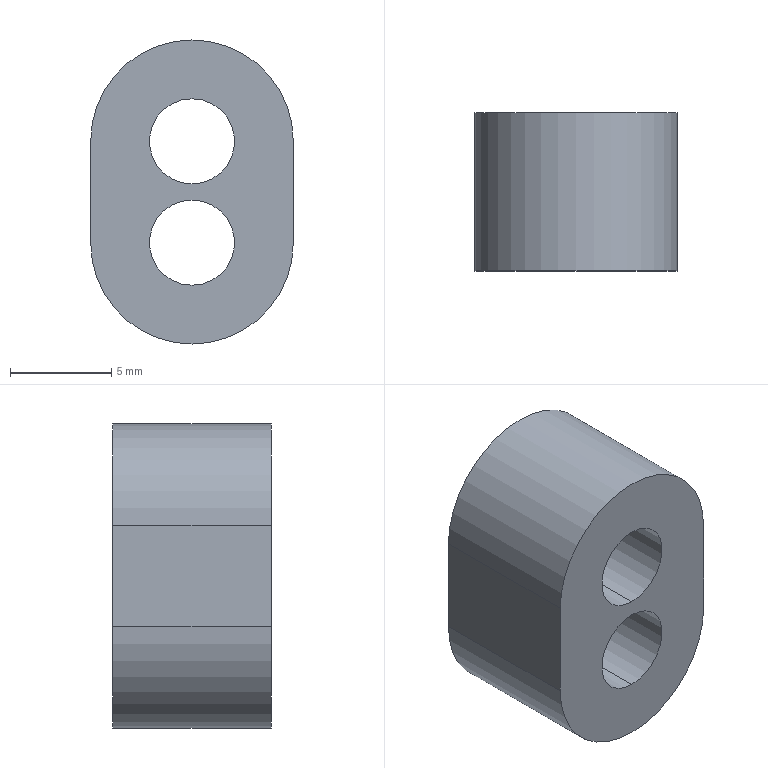Part | NX | features BREP 1 | 1 solid | 11 faces | box 10 x 7.8 x 15 mm | volume 786.482 mm3 | cylinder 7 | plane 4 | commonest cylinder face diameters 4.2 x4 10 x3
STEP:
#1=CARTESIAN_POINT('',(0.,7.8,0.4));
#2=VERTEX_POINT('',#1);
#3=CARTESIAN_POINT('',(0.,0.,0.4));
#4=VERTEX_POINT('',#3);
#5=CARTESIAN_POINT('',(0.,7.8,0.4));
#6=DIRECTION('',(0.,1.,0.));
#7=VECTOR('',#6,1000.);
#8=LINE('',#5,#7);
#9=EDGE_CURVE('',#2,#4,#8,.F.);
#10=ORIENTED_EDGE('',*,*,#9,.T.);
#11=CARTESIAN_POINT('',(0.,0.,4.6));
#12=VERTEX_POINT('',#11);
#13=CARTESIAN_POINT('',(0.,0.,2.5));
#14=DIRECTION('',(0.,1.,0.));
#15=DIRECTION('',(0.,0.,1.));
#16=AXIS2_PLACEMENT_3D('',#13,#14,#15);
#17=CIRCLE('',#16,2.1);
#18=EDGE_CURVE('',#12,#4,#17,.T.);
#19=ORIENTED_EDGE('',*,*,#18,.F.);
#20=CARTESIAN_POINT('',(0.,7.8,4.6));
#21=VERTEX_POINT('',#20);
#22=CARTESIAN_POINT('',(0.,7.8,4.6));
#23=DIRECTION('',(0.,1.,0.));
#24=VECTOR('',#23,1000.);
#25=LINE('',#22,#24);
#26=EDGE_CURVE('',#21,#12,#25,.F.);
#27=ORIENTED_EDGE('',*,*,#26,.F.);
#28=CARTESIAN_POINT('',(0.,7.8,2.5));
#29=DIRECTION('',(0.,1.,0.));
#30=DIRECTION('',(0.,0.,1.));
#31=AXIS2_PLACEMENT_3D('',#28,#29,#30);
#32=CIRCLE('',#31,2.1);
#33=EDGE_CURVE('',#21,#2,#32,.T.);
#34=ORIENTED_EDGE('',*,*,#33,.T.);
#35=EDGE_LOOP('',(#10,#19,#27,#34));
#36=FACE_BOUND('',#35,.T.);
#37=CARTESIAN_POINT('',(0.,7.8,2.5));
#38=DIRECTION('',(0.,1.,0.));
#39=DIRECTION('',(0.,0.,1.));
#40=AXIS2_PLACEMENT_3D('',#37,#38,#39);
#41=CYLINDRICAL_SURFACE('',#40,2.1);
#42=ADVANCED_FACE('',(#36),#41,.F.);
#43=CARTESIAN_POINT('',(0.,7.8,-4.6));
#44=VERTEX_POINT('',#43);
#45=CARTESIAN_POINT('',(0.,0.,-4.6));
#46=VERTEX_POINT('',#45);
#47=CARTESIAN_POINT('',(0.,7.8,-4.6));
#48=DIRECTION('',(0.,1.,0.));
#49=VECTOR('',#48,1000.);
#50=LINE('',#47,#49);
#51=EDGE_CURVE('',#44,#46,#50,.F.);
#52=ORIENTED_EDGE('',*,*,#51,.T.);
#53=CARTESIAN_POINT('',(0.,0.,-0.4));
#54=VERTEX_POINT('',#53);
#55=CARTESIAN_POINT('',(0.,0.,-2.5));
#56=DIRECTION('',(0.,1.,0.));
#57=DIRECTION('',(0.,0.,1.));
#58=AXIS2_PLACEMENT_3D('',#55,#56,#57);
#59=CIRCLE('',#58,2.1);
#60=EDGE_CURVE('',#54,#46,#59,.T.);
#61=ORIENTED_EDGE('',*,*,#60,.F.);
#62=CARTESIAN_POINT('',(0.,7.8,-0.4));
#63=VERTEX_POINT('',#62);
#64=CARTESIAN_POINT('',(0.,7.8,-0.4));
#65=DIRECTION('',(0.,1.,0.));
#66=VECTOR('',#65,1000.);
#67=LINE('',#64,#66);
#68=EDGE_CURVE('',#63,#54,#67,.F.);
#69=ORIENTED_EDGE('',*,*,#68,.F.);
#70=CARTESIAN_POINT('',(0.,7.8,-2.5));
#71=DIRECTION('',(0.,1.,0.));
#72=DIRECTION('',(0.,0.,1.));
#73=AXIS2_PLACEMENT_3D('',#70,#71,#72);
#74=CIRCLE('',#73,2.1);
#75=EDGE_CURVE('',#63,#44,#74,.T.);
#76=ORIENTED_EDGE('',*,*,#75,.T.);
#77=EDGE_LOOP('',(#52,#61,#69,#76));
#78=FACE_BOUND('',#77,.T.);
#79=CARTESIAN_POINT('',(0.,7.8,-2.5));
#80=DIRECTION('',(0.,1.,0.));
#81=DIRECTION('',(0.,0.,1.));
#82=AXIS2_PLACEMENT_3D('',#79,#80,#81);
#83=CYLINDRICAL_SURFACE('',#82,2.1);
#84=ADVANCED_FACE('',(#78),#83,.F.);
#85=CARTESIAN_POINT('',(-5.,0.,2.5));
#86=VERTEX_POINT('',#85);
#87=CARTESIAN_POINT('',(5.,0.,2.5));
#88=VERTEX_POINT('',#87);
#89=CARTESIAN_POINT('',(0.,0.,2.5));
#90=DIRECTION('',(0.,1.,0.));
#91=DIRECTION('',(0.,0.,1.));
#92=AXIS2_PLACEMENT_3D('',#89,#90,#91);
#93=CIRCLE('',#92,5.);
#94=EDGE_CURVE('',#86,#88,#93,.T.);
#95=ORIENTED_EDGE('',*,*,#94,.F.);
#96=CARTESIAN_POINT('',(-5.,0.,-2.5));
#97=VERTEX_POINT('',#96);
#98=CARTESIAN_POINT('',(-5.,0.,2.5));
#99=DIRECTION('',(0.,0.,1.));
#100=VECTOR('',#99,1000.);
#101=LINE('',#98,#100);
#102=EDGE_CURVE('',#97,#86,#101,.T.);
#103=ORIENTED_EDGE('',*,*,#102,.F.);
#104=CARTESIAN_POINT('',(0.,0.,-7.5));
#105=VERTEX_POINT('',#104);
#106=CARTESIAN_POINT('',(0.,0.,-2.5));
#107=DIRECTION('',(0.,1.,0.));
#108=DIRECTION('',(0.,0.,1.));
#109=AXIS2_PLACEMENT_3D('',#106,#107,#108);
#110=CIRCLE('',#109,5.);
#111=EDGE_CURVE('',#105,#97,#110,.T.);
#112=ORIENTED_EDGE('',*,*,#111,.F.);
#113=CARTESIAN_POINT('',(5.,0.,-2.5));
#114=VERTEX_POINT('',#113);
#115=CARTESIAN_POINT('',(0.,0.,-2.5));
#116=DIRECTION('',(0.,1.,0.));
#117=DIRECTION('',(0.,0.,1.));
#118=AXIS2_PLACEMENT_3D('',#115,#116,#117);
#119=CIRCLE('',#118,5.);
#120=EDGE_CURVE('',#114,#105,#119,.T.);
#121=ORIENTED_EDGE('',*,*,#120,.F.);
#122=CARTESIAN_POINT('',(5.,0.,2.5));
#123=DIRECTION('',(0.,0.,-1.));
#124=VECTOR('',#123,1000.);
#125=LINE('',#122,#124);
#126=EDGE_CURVE('',#88,#114,#125,.T.);
#127=ORIENTED_EDGE('',*,*,#126,.F.);
#128=EDGE_LOOP('',(#95,#103,#112,#121,#127));
#129=FACE_BOUND('',#128,.T.);
#130=ORIENTED_EDGE('',*,*,#60,.T.);
#131=CARTESIAN_POINT('',(0.,0.,-2.5));
#132=DIRECTION('',(0.,1.,0.));
#133=DIRECTION('',(0.,0.,1.));
#134=AXIS2_PLACEMENT_3D('',#131,#132,#133);
#135=CIRCLE('',#134,2.1);
#136=EDGE_CURVE('',#46,#54,#135,.T.);
#137=ORIENTED_EDGE('',*,*,#136,.T.);
#138=EDGE_LOOP('',(#130,#137));
#139=FACE_BOUND('',#138,.T.);
#140=ORIENTED_EDGE('',*,*,#18,.T.);
#141=CARTESIAN_POINT('',(0.,0.,2.5));
#142=DIRECTION('',(0.,1.,0.));
#143=DIRECTION('',(0.,0.,1.));
#144=AXIS2_PLACEMENT_3D('',#141,#142,#143);
#145=CIRCLE('',#144,2.1);
#146=EDGE_CURVE('',#4,#12,#145,.T.);
#147=ORIENTED_EDGE('',*,*,#146,.T.);
#148=EDGE_LOOP('',(#140,#147));
#149=FACE_BOUND('',#148,.T.);
#150=CARTESIAN_POINT('',(0.,0.,2.5));
#151=DIRECTION('',(0.,1.,0.));
#152=DIRECTION('',(0.,0.,1.));
#153=AXIS2_PLACEMENT_3D('',#150,#151,#152);
#154=PLANE('',#153);
#155=ADVANCED_FACE('',(#129,#139,#149),#154,.F.);
#156=CARTESIAN_POINT('',(-5.,7.8,2.5));
#157=VERTEX_POINT('',#156);
#158=CARTESIAN_POINT('',(5.,7.8,2.5));
#159=VERTEX_POINT('',#158);
#160=CARTESIAN_POINT('',(0.,7.8,2.5));
#161=DIRECTION('',(0.,1.,0.));
#162=DIRECTION('',(0.,0.,1.));
#163=AXIS2_PLACEMENT_3D('',#160,#161,#162);
#164=CIRCLE('',#163,5.);
#165=EDGE_CURVE('',#157,#159,#164,.T.);
#166=ORIENTED_EDGE('',*,*,#165,.T.);
#167=CARTESIAN_POINT('',(5.,7.8,-2.5));
#168=VERTEX_POINT('',#167);
#169=CARTESIAN_POINT('',(5.,7.8,2.5));
#170=DIRECTION('',(0.,0.,-1.));
#171=VECTOR('',#170,1000.);
#172=LINE('',#169,#171);
#173=EDGE_CURVE('',#159,#168,#172,.T.);
#174=ORIENTED_EDGE('',*,*,#173,.T.);
#175=CARTESIAN_POINT('',(0.,7.8,-7.5));
#176=VERTEX_POINT('',#175);
#177=CARTESIAN_POINT('',(0.,7.8,-2.5));
#178=DIRECTION('',(0.,1.,0.));
#179=DIRECTION('',(0.,0.,1.));
#180=AXIS2_PLACEMENT_3D('',#177,#178,#179);
#181=CIRCLE('',#180,5.);
#182=EDGE_CURVE('',#168,#176,#181,.T.);
#183=ORIENTED_EDGE('',*,*,#182,.T.);
#184=CARTESIAN_POINT('',(-5.,7.8,-2.5));
#185=VERTEX_POINT('',#184);
#186=CARTESIAN_POINT('',(0.,7.8,-2.5));
#187=DIRECTION('',(0.,1.,0.));
#188=DIRECTION('',(0.,0.,1.));
#189=AXIS2_PLACEMENT_3D('',#186,#187,#188);
#190=CIRCLE('',#189,5.);
#191=EDGE_CURVE('',#176,#185,#190,.T.);
#192=ORIENTED_EDGE('',*,*,#191,.T.);
#193=CARTESIAN_POINT('',(-5.,7.8,2.5));
#194=DIRECTION('',(0.,0.,1.));
#195=VECTOR('',#194,1000.);
#196=LINE('',#193,#195);
#197=EDGE_CURVE('',#185,#157,#196,.T.);
#198=ORIENTED_EDGE('',*,*,#197,.T.);
#199=EDGE_LOOP('',(#166,#174,#183,#192,#198));
#200=FACE_BOUND('',#199,.T.);
#201=ORIENTED_EDGE('',*,*,#75,.F.);
#202=CARTESIAN_POINT('',(0.,7.8,-2.5));
#203=DIRECTION('',(0.,1.,0.));
#204=DIRECTION('',(0.,0.,1.));
#205=AXIS2_PLACEMENT_3D('',#202,#203,#204);
#206=CIRCLE('',#205,2.1);
#207=EDGE_CURVE('',#44,#63,#206,.T.);
#208=ORIENTED_EDGE('',*,*,#207,.F.);
#209=EDGE_LOOP('',(#201,#208));
#210=FACE_BOUND('',#209,.T.);
#211=ORIENTED_EDGE('',*,*,#33,.F.);
#212=CARTESIAN_POINT('',(0.,7.8,2.5));
#213=DIRECTION('',(0.,1.,0.));
#214=DIRECTION('',(0.,0.,1.));
#215=AXIS2_PLACEMENT_3D('',#212,#213,#214);
#216=CIRCLE('',#215,2.1);
#217=EDGE_CURVE('',#2,#21,#216,.T.);
#218=ORIENTED_EDGE('',*,*,#217,.F.);
#219=EDGE_LOOP('',(#211,#218));
#220=FACE_BOUND('',#219,.T.);
#221=CARTESIAN_POINT('',(0.,7.8,2.5));
#222=DIRECTION('',(0.,1.,0.));
#223=DIRECTION('',(0.,0.,1.));
#224=AXIS2_PLACEMENT_3D('',#221,#222,#223);
#225=PLANE('',#224);
#226=ADVANCED_FACE('',(#200,#210,#220),#225,.T.);
#227=ORIENTED_EDGE('',*,*,#102,.T.);
#228=CARTESIAN_POINT('',(-5.,7.8,2.5));
#229=DIRECTION('',(0.,-1.,0.));
#230=VECTOR('',#229,1000.);
#231=LINE('',#228,#230);
#232=EDGE_CURVE('',#157,#86,#231,.T.);
#233=ORIENTED_EDGE('',*,*,#232,.F.);
#234=ORIENTED_EDGE('',*,*,#197,.F.);
#235=CARTESIAN_POINT('',(-5.,7.8,-2.5));
#236=DIRECTION('',(0.,-1.,0.));
#237=VECTOR('',#236,1000.);
#238=LINE('',#235,#237);
#239=EDGE_CURVE('',#185,#97,#238,.T.);
#240=ORIENTED_EDGE('',*,*,#239,.T.);
#241=EDGE_LOOP('',(#227,#233,#234,#240));
#242=FACE_BOUND('',#241,.T.);
#243=CARTESIAN_POINT('',(-5.,7.8,2.5));
#244=DIRECTION('',(1.,0.,0.));
#245=DIRECTION('',(0.,0.,-1.));
#246=AXIS2_PLACEMENT_3D('',#243,#244,#245);
#247=PLANE('',#246);
#248=ADVANCED_FACE('',(#242),#247,.F.);
#249=CARTESIAN_POINT('',(0.,7.8,-7.5));
#250=DIRECTION('',(0.,-1.,0.));
#251=VECTOR('',#250,1000.);
#252=LINE('',#249,#251);
#253=EDGE_CURVE('',#176,#105,#252,.T.);
#254=ORIENTED_EDGE('',*,*,#253,.F.);
#255=ORIENTED_EDGE('',*,*,#182,.F.);
#256=CARTESIAN_POINT('',(5.,7.8,-2.5));
#257=DIRECTION('',(0.,-1.,0.));
#258=VECTOR('',#257,1000.);
#259=LINE('',#256,#258);
#260=EDGE_CURVE('',#168,#114,#259,.T.);
#261=ORIENTED_EDGE('',*,*,#260,.T.);
#262=ORIENTED_EDGE('',*,*,#120,.T.);
#263=EDGE_LOOP('',(#254,#255,#261,#262));
#264=FACE_BOUND('',#263,.T.);
#265=CARTESIAN_POINT('',(0.,7.8,-2.5));
#266=DIRECTION('',(0.,-1.,0.));
#267=DIRECTION('',(0.,0.,-1.));
#268=AXIS2_PLACEMENT_3D('',#265,#266,#267);
#269=CYLINDRICAL_SURFACE('',#268,5.);
#270=ADVANCED_FACE('',(#264),#269,.T.);
#271=ORIENTED_EDGE('',*,*,#126,.T.);
#272=ORIENTED_EDGE('',*,*,#260,.F.);
#273=ORIENTED_EDGE('',*,*,#173,.F.);
#274=CARTESIAN_POINT('',(5.,7.8,2.5));
#275=DIRECTION('',(0.,-1.,0.));
#276=VECTOR('',#275,1000.);
#277=LINE('',#274,#276);
#278=EDGE_CURVE('',#159,#88,#277,.T.);
#279=ORIENTED_EDGE('',*,*,#278,.T.);
#280=EDGE_LOOP('',(#271,#272,#273,#279));
#281=FACE_BOUND('',#280,.T.);
#282=CARTESIAN_POINT('',(5.,7.8,2.5));
#283=DIRECTION('',(-1.,0.,0.));
#284=DIRECTION('',(0.,0.,1.));
#285=AXIS2_PLACEMENT_3D('',#282,#283,#284);
#286=PLANE('',#285);
#287=ADVANCED_FACE('',(#281),#286,.F.);
#288=ORIENTED_EDGE('',*,*,#94,.T.);
#289=ORIENTED_EDGE('',*,*,#278,.F.);
#290=ORIENTED_EDGE('',*,*,#165,.F.);
#291=ORIENTED_EDGE('',*,*,#232,.T.);
#292=EDGE_LOOP('',(#288,#289,#290,#291));
#293=FACE_BOUND('',#292,.T.);
#294=CARTESIAN_POINT('',(0.,7.8,2.5));
#295=DIRECTION('',(0.,-1.,0.));
#296=DIRECTION('',(0.,0.,-1.));
#297=AXIS2_PLACEMENT_3D('',#294,#295,#296);
#298=CYLINDRICAL_SURFACE('',#297,5.);
#299=ADVANCED_FACE('',(#293),#298,.T.);
#300=ORIENTED_EDGE('',*,*,#191,.F.);
#301=ORIENTED_EDGE('',*,*,#253,.T.);
#302=ORIENTED_EDGE('',*,*,#111,.T.);
#303=ORIENTED_EDGE('',*,*,#239,.F.);
#304=EDGE_LOOP('',(#300,#301,#302,#303));
#305=FACE_BOUND('',#304,.T.);
#306=CARTESIAN_POINT('',(0.,7.8,-2.5));
#307=DIRECTION('',(0.,-1.,0.));
#308=DIRECTION('',(0.,0.,-1.));
#309=AXIS2_PLACEMENT_3D('',#306,#307,#308);
#310=CYLINDRICAL_SURFACE('',#309,5.);
#311=ADVANCED_FACE('',(#305),#310,.T.);
#312=ORIENTED_EDGE('',*,*,#136,.F.);
#313=ORIENTED_EDGE('',*,*,#51,.F.);
#314=ORIENTED_EDGE('',*,*,#207,.T.);
#315=ORIENTED_EDGE('',*,*,#68,.T.);
#316=EDGE_LOOP('',(#312,#313,#314,#315));
#317=FACE_BOUND('',#316,.T.);
#318=CARTESIAN_POINT('',(0.,7.8,-2.5));
#319=DIRECTION('',(0.,1.,0.));
#320=DIRECTION('',(0.,0.,1.));
#321=AXIS2_PLACEMENT_3D('',#318,#319,#320);
#322=CYLINDRICAL_SURFACE('',#321,2.1);
#323=ADVANCED_FACE('',(#317),#322,.F.);
#324=ORIENTED_EDGE('',*,*,#146,.F.);
#325=ORIENTED_EDGE('',*,*,#9,.F.);
#326=ORIENTED_EDGE('',*,*,#217,.T.);
#327=ORIENTED_EDGE('',*,*,#26,.T.);
#328=EDGE_LOOP('',(#324,#325,#326,#327));
#329=FACE_BOUND('',#328,.T.);
#330=CARTESIAN_POINT('',(0.,7.8,2.5));
#331=DIRECTION('',(0.,1.,0.));
#332=DIRECTION('',(0.,0.,1.));
#333=AXIS2_PLACEMENT_3D('',#330,#331,#332);
#334=CYLINDRICAL_SURFACE('',#333,2.1);
#335=ADVANCED_FACE('',(#329),#334,.F.);
#336=CLOSED_SHELL('',(#42,#84,#155,#226,#248,#270,#287,#299,#311,#323,#335));
#337=MANIFOLD_SOLID_BREP('',#336);
#338=(LENGTH_UNIT()NAMED_UNIT(*)SI_UNIT(.MILLI.,.METRE.));
#339=UNCERTAINTY_MEASURE_WITH_UNIT(LENGTH_MEASURE(0.00001),#338,'','');
#340=(NAMED_UNIT(*)PLANE_ANGLE_UNIT()SI_UNIT($,.RADIAN.));
#341=(NAMED_UNIT(*)SI_UNIT($,.STERADIAN.)SOLID_ANGLE_UNIT());
#342=(GEOMETRIC_REPRESENTATION_CONTEXT(3)GLOBAL_UNCERTAINTY_ASSIGNED_CONTEXT((#339))GLOBAL_UNIT_ASSIGNED_CONTEXT((#338,#340,#341))REPRESENTATION_CONTEXT('',''));
#343=ADVANCED_BREP_SHAPE_REPRESENTATION('',(#337),#342);